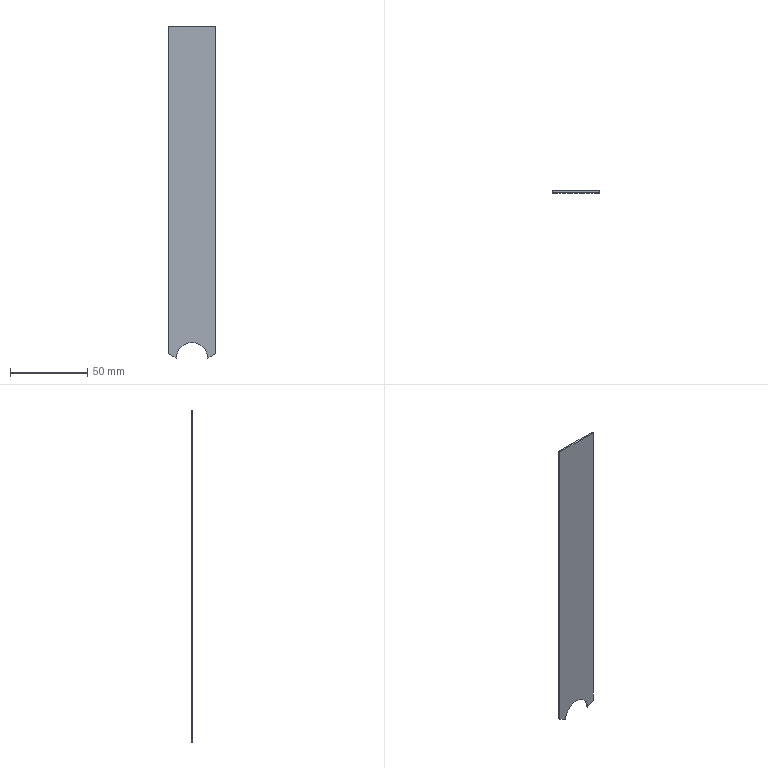Part | STEP file | solid 162 | 1 solid | 10 faces | box 30.5 x 1 x 214.425 mm | volume 6372 mm3 | plane 5 | cylinder 3 | cone 2 | commonest cylinder face diameters 30.5 x2 20 x1